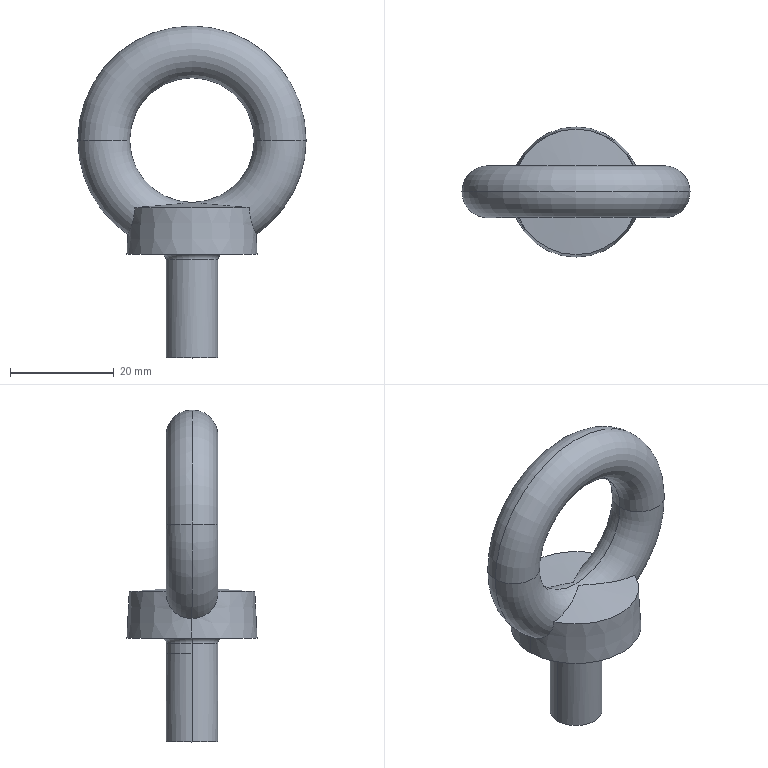Part | NX | features solid 2 | 1 solid | 18 faces | box 44 x 25.1 x 64 mm | volume 12780 mm3 | torus 6 | cylinder 4 | cone 4 | plane 2 | sphere 2 | commonest cylinder face diameters 10 x4